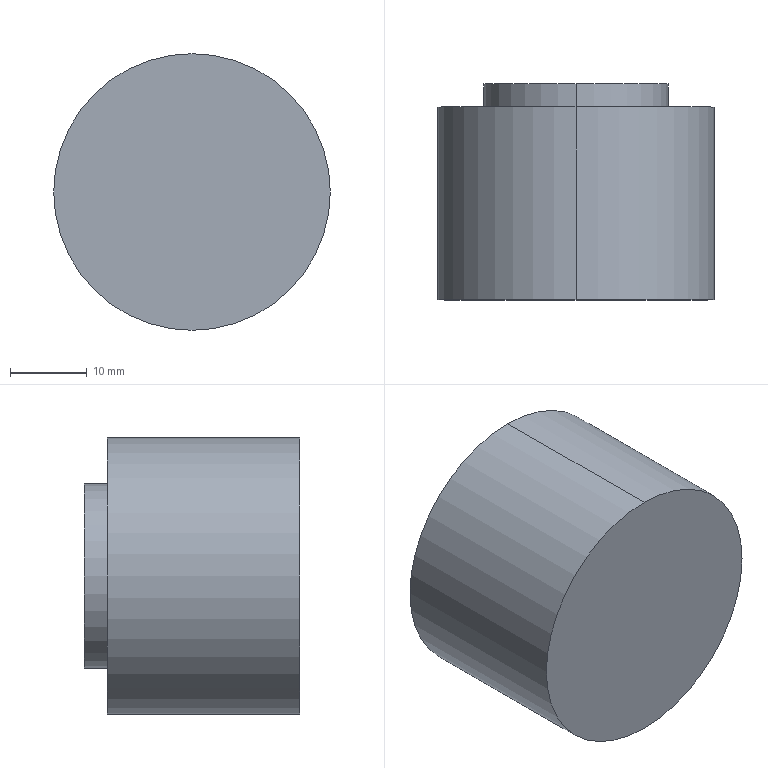Part | SolidWorks | features Extrusion 1, ICE 1 | 1 solid | 7 faces | box 36 x 28.1 x 36 mm | volume 26906 mm3 | cylinder 4 | plane 3 | commonest cylinder face diameters 24 x2 36 x2
STEP:
#1=CARTESIAN_POINT('',(0.,28.1,12.));
#2=VERTEX_POINT('',#1);
#3=CARTESIAN_POINT('',(0.,28.1,-12.));
#4=VERTEX_POINT('',#3);
#5=CARTESIAN_POINT('',(0.,28.1,0.));
#6=DIRECTION('',(0.,1.,0.));
#7=DIRECTION('',(0.,0.,1.));
#8=AXIS2_PLACEMENT_3D('',#5,#6,#7);
#9=CIRCLE('',#8,12.);
#10=EDGE_CURVE('',#2,#4,#9,.T.);
#11=ORIENTED_EDGE('',*,*,#10,.F.);
#12=CARTESIAN_POINT('',(0.,25.1,12.));
#13=VERTEX_POINT('',#12);
#14=CARTESIAN_POINT('',(0.,28.1,12.));
#15=DIRECTION('',(0.,-1.,0.));
#16=VECTOR('',#15,1000.);
#17=LINE('',#14,#16);
#18=EDGE_CURVE('',#2,#13,#17,.T.);
#19=ORIENTED_EDGE('',*,*,#18,.T.);
#20=CARTESIAN_POINT('',(0.,25.1,-12.));
#21=VERTEX_POINT('',#20);
#22=CARTESIAN_POINT('',(0.,25.1,0.));
#23=DIRECTION('',(0.,1.,0.));
#24=DIRECTION('',(0.,0.,1.));
#25=AXIS2_PLACEMENT_3D('',#22,#23,#24);
#26=CIRCLE('',#25,12.);
#27=EDGE_CURVE('',#13,#21,#26,.T.);
#28=ORIENTED_EDGE('',*,*,#27,.T.);
#29=CARTESIAN_POINT('',(0.,28.1,-12.));
#30=DIRECTION('',(0.,-1.,0.));
#31=VECTOR('',#30,1000.);
#32=LINE('',#29,#31);
#33=EDGE_CURVE('',#4,#21,#32,.T.);
#34=ORIENTED_EDGE('',*,*,#33,.F.);
#35=EDGE_LOOP('',(#11,#19,#28,#34));
#36=FACE_OUTER_BOUND('',#35,.T.);
#37=CARTESIAN_POINT('',(0.,28.1,0.));
#38=DIRECTION('',(0.,-1.,0.));
#39=DIRECTION('',(0.,0.,-1.));
#40=AXIS2_PLACEMENT_3D('',#37,#38,#39);
#41=CYLINDRICAL_SURFACE('',#40,12.);
#42=ADVANCED_FACE('',(#36),#41,.T.);
#43=CARTESIAN_POINT('',(0.,25.1,18.));
#44=VERTEX_POINT('',#43);
#45=CARTESIAN_POINT('',(0.,25.1,-18.));
#46=VERTEX_POINT('',#45);
#47=CARTESIAN_POINT('',(0.,25.1,0.));
#48=DIRECTION('',(0.,1.,0.));
#49=DIRECTION('',(0.,0.,1.));
#50=AXIS2_PLACEMENT_3D('',#47,#48,#49);
#51=CIRCLE('',#50,18.);
#52=EDGE_CURVE('',#44,#46,#51,.T.);
#53=ORIENTED_EDGE('',*,*,#52,.F.);
#54=CARTESIAN_POINT('',(0.,0.,18.));
#55=VERTEX_POINT('',#54);
#56=CARTESIAN_POINT('',(0.,25.1,18.));
#57=DIRECTION('',(0.,-1.,0.));
#58=VECTOR('',#57,1000.);
#59=LINE('',#56,#58);
#60=EDGE_CURVE('',#44,#55,#59,.T.);
#61=ORIENTED_EDGE('',*,*,#60,.T.);
#62=CARTESIAN_POINT('',(0.,0.,-18.));
#63=VERTEX_POINT('',#62);
#64=CARTESIAN_POINT('',(0.,0.,0.));
#65=DIRECTION('',(0.,1.,0.));
#66=DIRECTION('',(0.,0.,1.));
#67=AXIS2_PLACEMENT_3D('',#64,#65,#66);
#68=CIRCLE('',#67,18.);
#69=EDGE_CURVE('',#55,#63,#68,.T.);
#70=ORIENTED_EDGE('',*,*,#69,.T.);
#71=CARTESIAN_POINT('',(0.,25.1,-18.));
#72=DIRECTION('',(0.,-1.,0.));
#73=VECTOR('',#72,1000.);
#74=LINE('',#71,#73);
#75=EDGE_CURVE('',#46,#63,#74,.T.);
#76=ORIENTED_EDGE('',*,*,#75,.F.);
#77=EDGE_LOOP('',(#53,#61,#70,#76));
#78=FACE_OUTER_BOUND('',#77,.T.);
#79=CARTESIAN_POINT('',(0.,25.1,0.));
#80=DIRECTION('',(0.,-1.,0.));
#81=DIRECTION('',(0.,0.,-1.));
#82=AXIS2_PLACEMENT_3D('',#79,#80,#81);
#83=CYLINDRICAL_SURFACE('',#82,18.);
#84=ADVANCED_FACE('',(#78),#83,.T.);
#85=ORIENTED_EDGE('',*,*,#60,.F.);
#86=CARTESIAN_POINT('',(0.,25.1,0.));
#87=DIRECTION('',(0.,1.,0.));
#88=DIRECTION('',(0.,0.,1.));
#89=AXIS2_PLACEMENT_3D('',#86,#87,#88);
#90=CIRCLE('',#89,18.);
#91=EDGE_CURVE('',#46,#44,#90,.T.);
#92=ORIENTED_EDGE('',*,*,#91,.F.);
#93=ORIENTED_EDGE('',*,*,#75,.T.);
#94=CARTESIAN_POINT('',(0.,0.,0.));
#95=DIRECTION('',(0.,1.,0.));
#96=DIRECTION('',(0.,0.,1.));
#97=AXIS2_PLACEMENT_3D('',#94,#95,#96);
#98=CIRCLE('',#97,18.);
#99=EDGE_CURVE('',#63,#55,#98,.T.);
#100=ORIENTED_EDGE('',*,*,#99,.T.);
#101=EDGE_LOOP('',(#85,#92,#93,#100));
#102=FACE_OUTER_BOUND('',#101,.T.);
#103=CARTESIAN_POINT('',(0.,25.1,0.));
#104=DIRECTION('',(0.,-1.,0.));
#105=DIRECTION('',(0.,0.,-1.));
#106=AXIS2_PLACEMENT_3D('',#103,#104,#105);
#107=CYLINDRICAL_SURFACE('',#106,18.);
#108=ADVANCED_FACE('',(#102),#107,.T.);
#109=CARTESIAN_POINT('',(0.,25.1,0.));
#110=DIRECTION('',(0.,1.,0.));
#111=DIRECTION('',(0.,0.,1.));
#112=AXIS2_PLACEMENT_3D('',#109,#110,#111);
#113=CIRCLE('',#112,12.);
#114=EDGE_CURVE('',#21,#13,#113,.T.);
#115=ORIENTED_EDGE('',*,*,#114,.F.);
#116=ORIENTED_EDGE('',*,*,#27,.F.);
#117=EDGE_LOOP('',(#115,#116));
#118=FACE_BOUND('',#117,.T.);
#119=ORIENTED_EDGE('',*,*,#91,.T.);
#120=ORIENTED_EDGE('',*,*,#52,.T.);
#121=EDGE_LOOP('',(#119,#120));
#122=FACE_OUTER_BOUND('',#121,.T.);
#123=CARTESIAN_POINT('',(0.,25.1,0.));
#124=DIRECTION('',(0.,1.,0.));
#125=DIRECTION('',(0.,0.,1.));
#126=AXIS2_PLACEMENT_3D('',#123,#124,#125);
#127=PLANE('',#126);
#128=ADVANCED_FACE('',(#118,#122),#127,.T.);
#129=ORIENTED_EDGE('',*,*,#99,.F.);
#130=ORIENTED_EDGE('',*,*,#69,.F.);
#131=EDGE_LOOP('',(#129,#130));
#132=FACE_OUTER_BOUND('',#131,.T.);
#133=CARTESIAN_POINT('',(0.,0.,0.));
#134=DIRECTION('',(0.,1.,0.));
#135=DIRECTION('',(0.,0.,1.));
#136=AXIS2_PLACEMENT_3D('',#133,#134,#135);
#137=PLANE('',#136);
#138=ADVANCED_FACE('',(#132),#137,.F.);
#139=ORIENTED_EDGE('',*,*,#18,.F.);
#140=CARTESIAN_POINT('',(0.,28.1,0.));
#141=DIRECTION('',(0.,1.,0.));
#142=DIRECTION('',(0.,0.,1.));
#143=AXIS2_PLACEMENT_3D('',#140,#141,#142);
#144=CIRCLE('',#143,12.);
#145=EDGE_CURVE('',#4,#2,#144,.T.);
#146=ORIENTED_EDGE('',*,*,#145,.F.);
#147=ORIENTED_EDGE('',*,*,#33,.T.);
#148=ORIENTED_EDGE('',*,*,#114,.T.);
#149=EDGE_LOOP('',(#139,#146,#147,#148));
#150=FACE_OUTER_BOUND('',#149,.T.);
#151=CARTESIAN_POINT('',(0.,28.1,0.));
#152=DIRECTION('',(0.,-1.,0.));
#153=DIRECTION('',(0.,0.,-1.));
#154=AXIS2_PLACEMENT_3D('',#151,#152,#153);
#155=CYLINDRICAL_SURFACE('',#154,12.);
#156=ADVANCED_FACE('',(#150),#155,.T.);
#157=ORIENTED_EDGE('',*,*,#145,.T.);
#158=ORIENTED_EDGE('',*,*,#10,.T.);
#159=EDGE_LOOP('',(#157,#158));
#160=FACE_OUTER_BOUND('',#159,.T.);
#161=CARTESIAN_POINT('',(0.,28.1,0.));
#162=DIRECTION('',(0.,1.,0.));
#163=DIRECTION('',(0.,0.,1.));
#164=AXIS2_PLACEMENT_3D('',#161,#162,#163);
#165=PLANE('',#164);
#166=ADVANCED_FACE('',(#160),#165,.T.);
#167=CLOSED_SHELL('',(#42,#84,#108,#128,#138,#156,#166));
#168=MANIFOLD_SOLID_BREP('',#167);
#169=CARTESIAN_POINT('',(0.,0.,0.));
#170=DIRECTION('',(0.,0.,1.));
#171=DIRECTION('',(1.,0.,0.));
#172=AXIS2_PLACEMENT_3D('',#169,#170,#171);
#173=(LENGTH_UNIT()NAMED_UNIT(*)SI_UNIT(.MILLI.,.METRE.));
#174=UNCERTAINTY_MEASURE_WITH_UNIT(LENGTH_MEASURE(0.00001),#173,'','');
#175=(NAMED_UNIT(*)PLANE_ANGLE_UNIT()SI_UNIT($,.RADIAN.));
#176=(NAMED_UNIT(*)SI_UNIT($,.STERADIAN.)SOLID_ANGLE_UNIT());
#177=(GEOMETRIC_REPRESENTATION_CONTEXT(3)GLOBAL_UNCERTAINTY_ASSIGNED_CONTEXT((#174))GLOBAL_UNIT_ASSIGNED_CONTEXT((#173,#175,#176))REPRESENTATION_CONTEXT('',''));
#178=ADVANCED_BREP_SHAPE_REPRESENTATION('',(#168,#172),#177);